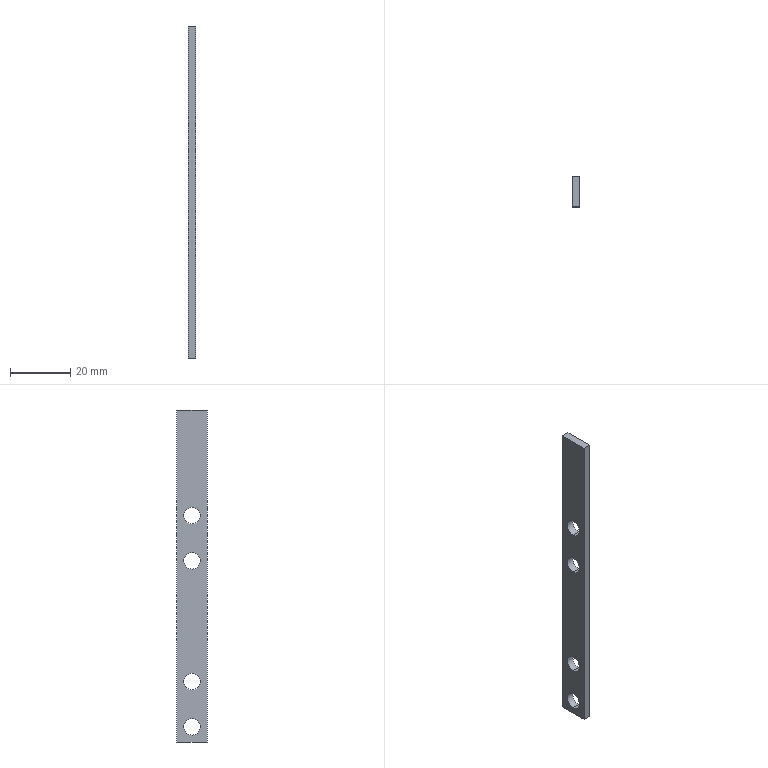Part | SolidWorks | features BaseBody 1 | 1 solid | 14 faces | box 2.5 x 10 x 110 mm | volume 2512 mm3 | cylinder 8 | plane 6 | commonest cylinder face diameters 5.5 x8
STEP:
#1=CARTESIAN_POINT('',(944.446,-4365.973,912.221));
#2=VERTEX_POINT('',#1);
#3=CARTESIAN_POINT('',(944.446,-4365.973,917.721));
#4=VERTEX_POINT('',#3);
#5=CARTESIAN_POINT('',(944.446,-4365.973,914.971));
#6=DIRECTION('',(-1.,0.,0.));
#7=DIRECTION('',(0.,0.,1.));
#8=AXIS2_PLACEMENT_3D('',#5,#6,#7);
#9=CIRCLE('',#8,2.75);
#10=EDGE_CURVE('',#2,#4,#9,.T.);
#11=ORIENTED_EDGE('',*,*,#10,.F.);
#12=CARTESIAN_POINT('',(941.946,-4365.973,912.221));
#13=VERTEX_POINT('',#12);
#14=CARTESIAN_POINT('',(882.499,-4365.973,912.221));
#15=DIRECTION('',(-1.,0.,0.));
#16=VECTOR('',#15,1000.);
#17=LINE('',#14,#16);
#18=EDGE_CURVE('',#2,#13,#17,.T.);
#19=ORIENTED_EDGE('',*,*,#18,.T.);
#20=CARTESIAN_POINT('',(941.946,-4365.973,917.721));
#21=VERTEX_POINT('',#20);
#22=CARTESIAN_POINT('',(941.946,-4365.973,914.971));
#23=DIRECTION('',(1.,0.,0.));
#24=DIRECTION('',(0.,0.,1.));
#25=AXIS2_PLACEMENT_3D('',#22,#23,#24);
#26=CIRCLE('',#25,2.75);
#27=EDGE_CURVE('',#21,#13,#26,.T.);
#28=ORIENTED_EDGE('',*,*,#27,.F.);
#29=CARTESIAN_POINT('',(882.499,-4365.973,917.721));
#30=DIRECTION('',(-1.,0.,0.));
#31=VECTOR('',#30,1000.);
#32=LINE('',#29,#31);
#33=EDGE_CURVE('',#4,#21,#32,.T.);
#34=ORIENTED_EDGE('',*,*,#33,.F.);
#35=EDGE_LOOP('',(#11,#19,#28,#34));
#36=FACE_OUTER_BOUND('',#35,.T.);
#37=CARTESIAN_POINT('',(882.499,-4365.973,914.971));
#38=DIRECTION('',(-1.,0.,0.));
#39=DIRECTION('',(0.,0.,1.));
#40=AXIS2_PLACEMENT_3D('',#37,#38,#39);
#41=CYLINDRICAL_SURFACE('',#40,2.75);
#42=ADVANCED_FACE('',(#36),#41,.F.);
#43=CARTESIAN_POINT('',(941.946,-4365.973,877.721));
#44=VERTEX_POINT('',#43);
#45=CARTESIAN_POINT('',(941.946,-4365.973,872.221));
#46=VERTEX_POINT('',#45);
#47=CARTESIAN_POINT('',(941.946,-4365.973,874.971));
#48=DIRECTION('',(1.,0.,0.));
#49=DIRECTION('',(0.,0.,-1.));
#50=AXIS2_PLACEMENT_3D('',#47,#48,#49);
#51=CIRCLE('',#50,2.75);
#52=EDGE_CURVE('',#44,#46,#51,.T.);
#53=ORIENTED_EDGE('',*,*,#52,.F.);
#54=CARTESIAN_POINT('',(944.446,-4365.973,877.721));
#55=VERTEX_POINT('',#54);
#56=CARTESIAN_POINT('',(882.499,-4365.973,877.721));
#57=DIRECTION('',(1.,0.,0.));
#58=VECTOR('',#57,1000.);
#59=LINE('',#56,#58);
#60=EDGE_CURVE('',#44,#55,#59,.T.);
#61=ORIENTED_EDGE('',*,*,#60,.T.);
#62=CARTESIAN_POINT('',(944.446,-4365.973,872.221));
#63=VERTEX_POINT('',#62);
#64=CARTESIAN_POINT('',(944.446,-4365.973,874.971));
#65=DIRECTION('',(-1.,0.,0.));
#66=DIRECTION('',(0.,0.,-1.));
#67=AXIS2_PLACEMENT_3D('',#64,#65,#66);
#68=CIRCLE('',#67,2.75);
#69=EDGE_CURVE('',#63,#55,#68,.T.);
#70=ORIENTED_EDGE('',*,*,#69,.F.);
#71=CARTESIAN_POINT('',(882.499,-4365.973,872.221));
#72=DIRECTION('',(1.,0.,0.));
#73=VECTOR('',#72,1000.);
#74=LINE('',#71,#73);
#75=EDGE_CURVE('',#46,#63,#74,.T.);
#76=ORIENTED_EDGE('',*,*,#75,.F.);
#77=EDGE_LOOP('',(#53,#61,#70,#76));
#78=FACE_OUTER_BOUND('',#77,.T.);
#79=CARTESIAN_POINT('',(882.499,-4365.973,874.971));
#80=DIRECTION('',(1.,0.,0.));
#81=DIRECTION('',(0.,0.,-1.));
#82=AXIS2_PLACEMENT_3D('',#79,#80,#81);
#83=CYLINDRICAL_SURFACE('',#82,2.75);
#84=ADVANCED_FACE('',(#78),#83,.F.);
#85=CARTESIAN_POINT('',(941.946,-4365.973,862.721));
#86=VERTEX_POINT('',#85);
#87=CARTESIAN_POINT('',(941.946,-4365.973,857.221));
#88=VERTEX_POINT('',#87);
#89=CARTESIAN_POINT('',(941.946,-4365.973,859.971));
#90=DIRECTION('',(1.,0.,0.));
#91=DIRECTION('',(0.,0.,-1.));
#92=AXIS2_PLACEMENT_3D('',#89,#90,#91);
#93=CIRCLE('',#92,2.75);
#94=EDGE_CURVE('',#86,#88,#93,.T.);
#95=ORIENTED_EDGE('',*,*,#94,.F.);
#96=CARTESIAN_POINT('',(944.446,-4365.973,862.721));
#97=VERTEX_POINT('',#96);
#98=CARTESIAN_POINT('',(882.499,-4365.973,862.721));
#99=DIRECTION('',(1.,0.,0.));
#100=VECTOR('',#99,1000.);
#101=LINE('',#98,#100);
#102=EDGE_CURVE('',#86,#97,#101,.T.);
#103=ORIENTED_EDGE('',*,*,#102,.T.);
#104=CARTESIAN_POINT('',(944.446,-4365.973,857.221));
#105=VERTEX_POINT('',#104);
#106=CARTESIAN_POINT('',(944.446,-4365.973,859.971));
#107=DIRECTION('',(-1.,0.,0.));
#108=DIRECTION('',(0.,0.,-1.));
#109=AXIS2_PLACEMENT_3D('',#106,#107,#108);
#110=CIRCLE('',#109,2.75);
#111=EDGE_CURVE('',#105,#97,#110,.T.);
#112=ORIENTED_EDGE('',*,*,#111,.F.);
#113=CARTESIAN_POINT('',(882.499,-4365.973,857.221));
#114=DIRECTION('',(1.,0.,0.));
#115=VECTOR('',#114,1000.);
#116=LINE('',#113,#115);
#117=EDGE_CURVE('',#88,#105,#116,.T.);
#118=ORIENTED_EDGE('',*,*,#117,.F.);
#119=EDGE_LOOP('',(#95,#103,#112,#118));
#120=FACE_OUTER_BOUND('',#119,.T.);
#121=CARTESIAN_POINT('',(882.499,-4365.973,859.971));
#122=DIRECTION('',(1.,0.,0.));
#123=DIRECTION('',(0.,0.,-1.));
#124=AXIS2_PLACEMENT_3D('',#121,#122,#123);
#125=CYLINDRICAL_SURFACE('',#124,2.75);
#126=ADVANCED_FACE('',(#120),#125,.F.);
#127=CARTESIAN_POINT('',(944.446,-4365.973,927.221));
#128=VERTEX_POINT('',#127);
#129=CARTESIAN_POINT('',(944.446,-4365.973,932.721));
#130=VERTEX_POINT('',#129);
#131=CARTESIAN_POINT('',(944.446,-4365.973,929.971));
#132=DIRECTION('',(-1.,0.,0.));
#133=DIRECTION('',(0.,0.,1.));
#134=AXIS2_PLACEMENT_3D('',#131,#132,#133);
#135=CIRCLE('',#134,2.75);
#136=EDGE_CURVE('',#128,#130,#135,.T.);
#137=ORIENTED_EDGE('',*,*,#136,.F.);
#138=CARTESIAN_POINT('',(941.946,-4365.973,927.221));
#139=VERTEX_POINT('',#138);
#140=CARTESIAN_POINT('',(882.499,-4365.973,927.221));
#141=DIRECTION('',(-1.,0.,0.));
#142=VECTOR('',#141,1000.);
#143=LINE('',#140,#142);
#144=EDGE_CURVE('',#128,#139,#143,.T.);
#145=ORIENTED_EDGE('',*,*,#144,.T.);
#146=CARTESIAN_POINT('',(941.946,-4365.973,932.721));
#147=VERTEX_POINT('',#146);
#148=CARTESIAN_POINT('',(941.946,-4365.973,929.971));
#149=DIRECTION('',(1.,0.,0.));
#150=DIRECTION('',(0.,0.,1.));
#151=AXIS2_PLACEMENT_3D('',#148,#149,#150);
#152=CIRCLE('',#151,2.75);
#153=EDGE_CURVE('',#147,#139,#152,.T.);
#154=ORIENTED_EDGE('',*,*,#153,.F.);
#155=CARTESIAN_POINT('',(882.499,-4365.973,932.721));
#156=DIRECTION('',(-1.,0.,0.));
#157=VECTOR('',#156,1000.);
#158=LINE('',#155,#157);
#159=EDGE_CURVE('',#130,#147,#158,.T.);
#160=ORIENTED_EDGE('',*,*,#159,.F.);
#161=EDGE_LOOP('',(#137,#145,#154,#160));
#162=FACE_OUTER_BOUND('',#161,.T.);
#163=CARTESIAN_POINT('',(882.499,-4365.973,929.971));
#164=DIRECTION('',(-1.,0.,0.));
#165=DIRECTION('',(0.,0.,1.));
#166=AXIS2_PLACEMENT_3D('',#163,#164,#165);
#167=CYLINDRICAL_SURFACE('',#166,2.75);
#168=ADVANCED_FACE('',(#162),#167,.F.);
#169=CARTESIAN_POINT('',(941.946,-4360.973,854.971));
#170=VERTEX_POINT('',#169);
#171=CARTESIAN_POINT('',(941.946,-4370.973,854.971));
#172=VERTEX_POINT('',#171);
#173=CARTESIAN_POINT('',(941.946,-4370.973,854.971));
#174=DIRECTION('',(0.,-1.,0.));
#175=VECTOR('',#174,1000.);
#176=LINE('',#173,#175);
#177=EDGE_CURVE('',#170,#172,#176,.T.);
#178=ORIENTED_EDGE('',*,*,#177,.T.);
#179=CARTESIAN_POINT('',(941.946,-4370.973,964.971));
#180=VERTEX_POINT('',#179);
#181=CARTESIAN_POINT('',(941.946,-4370.973,854.971));
#182=DIRECTION('',(0.,0.,1.));
#183=VECTOR('',#182,1000.);
#184=LINE('',#181,#183);
#185=EDGE_CURVE('',#172,#180,#184,.T.);
#186=ORIENTED_EDGE('',*,*,#185,.T.);
#187=CARTESIAN_POINT('',(941.946,-4360.973,964.971));
#188=VERTEX_POINT('',#187);
#189=CARTESIAN_POINT('',(941.946,-4370.973,964.971));
#190=DIRECTION('',(0.,1.,0.));
#191=VECTOR('',#190,1000.);
#192=LINE('',#189,#191);
#193=EDGE_CURVE('',#180,#188,#192,.T.);
#194=ORIENTED_EDGE('',*,*,#193,.T.);
#195=CARTESIAN_POINT('',(941.946,-4360.973,854.971));
#196=DIRECTION('',(0.,0.,-1.));
#197=VECTOR('',#196,1000.);
#198=LINE('',#195,#197);
#199=EDGE_CURVE('',#188,#170,#198,.T.);
#200=ORIENTED_EDGE('',*,*,#199,.T.);
#201=EDGE_LOOP('',(#178,#186,#194,#200));
#202=FACE_OUTER_BOUND('',#201,.T.);
#203=ORIENTED_EDGE('',*,*,#27,.T.);
#204=CARTESIAN_POINT('',(941.946,-4365.973,914.971));
#205=DIRECTION('',(1.,0.,0.));
#206=DIRECTION('',(0.,0.,1.));
#207=AXIS2_PLACEMENT_3D('',#204,#205,#206);
#208=CIRCLE('',#207,2.75);
#209=EDGE_CURVE('',#13,#21,#208,.T.);
#210=ORIENTED_EDGE('',*,*,#209,.T.);
#211=EDGE_LOOP('',(#203,#210));
#212=FACE_BOUND('',#211,.T.);
#213=CARTESIAN_POINT('',(941.946,-4365.973,874.971));
#214=DIRECTION('',(1.,0.,0.));
#215=DIRECTION('',(0.,0.,-1.));
#216=AXIS2_PLACEMENT_3D('',#213,#214,#215);
#217=CIRCLE('',#216,2.75);
#218=EDGE_CURVE('',#46,#44,#217,.T.);
#219=ORIENTED_EDGE('',*,*,#218,.T.);
#220=ORIENTED_EDGE('',*,*,#52,.T.);
#221=EDGE_LOOP('',(#219,#220));
#222=FACE_BOUND('',#221,.T.);
#223=CARTESIAN_POINT('',(941.946,-4365.973,859.971));
#224=DIRECTION('',(1.,0.,0.));
#225=DIRECTION('',(0.,0.,-1.));
#226=AXIS2_PLACEMENT_3D('',#223,#224,#225);
#227=CIRCLE('',#226,2.75);
#228=EDGE_CURVE('',#88,#86,#227,.T.);
#229=ORIENTED_EDGE('',*,*,#228,.T.);
#230=ORIENTED_EDGE('',*,*,#94,.T.);
#231=EDGE_LOOP('',(#229,#230));
#232=FACE_BOUND('',#231,.T.);
#233=ORIENTED_EDGE('',*,*,#153,.T.);
#234=CARTESIAN_POINT('',(941.946,-4365.973,929.971));
#235=DIRECTION('',(1.,0.,0.));
#236=DIRECTION('',(0.,0.,1.));
#237=AXIS2_PLACEMENT_3D('',#234,#235,#236);
#238=CIRCLE('',#237,2.75);
#239=EDGE_CURVE('',#139,#147,#238,.T.);
#240=ORIENTED_EDGE('',*,*,#239,.T.);
#241=EDGE_LOOP('',(#233,#240));
#242=FACE_BOUND('',#241,.T.);
#243=CARTESIAN_POINT('',(941.946,-4370.973,854.971));
#244=DIRECTION('',(-1.,0.,0.));
#245=DIRECTION('',(0.,0.,1.));
#246=AXIS2_PLACEMENT_3D('',#243,#244,#245);
#247=PLANE('',#246);
#248=ADVANCED_FACE('',(#202,#212,#222,#232,#242),#247,.T.);
#249=CARTESIAN_POINT('',(944.446,-4370.973,854.971));
#250=VERTEX_POINT('',#249);
#251=CARTESIAN_POINT('',(944.446,-4370.973,854.971));
#252=DIRECTION('',(1.,0.,0.));
#253=VECTOR('',#252,1000.);
#254=LINE('',#251,#253);
#255=EDGE_CURVE('',#172,#250,#254,.T.);
#256=ORIENTED_EDGE('',*,*,#255,.T.);
#257=CARTESIAN_POINT('',(944.446,-4370.973,964.971));
#258=VERTEX_POINT('',#257);
#259=CARTESIAN_POINT('',(944.446,-4370.973,854.971));
#260=DIRECTION('',(0.,0.,1.));
#261=VECTOR('',#260,1000.);
#262=LINE('',#259,#261);
#263=EDGE_CURVE('',#250,#258,#262,.T.);
#264=ORIENTED_EDGE('',*,*,#263,.T.);
#265=CARTESIAN_POINT('',(944.446,-4370.973,964.971));
#266=DIRECTION('',(-1.,0.,0.));
#267=VECTOR('',#266,1000.);
#268=LINE('',#265,#267);
#269=EDGE_CURVE('',#258,#180,#268,.T.);
#270=ORIENTED_EDGE('',*,*,#269,.T.);
#271=ORIENTED_EDGE('',*,*,#185,.F.);
#272=EDGE_LOOP('',(#256,#264,#270,#271));
#273=FACE_OUTER_BOUND('',#272,.T.);
#274=CARTESIAN_POINT('',(944.446,-4370.973,854.971));
#275=DIRECTION('',(0.,-1.,0.));
#276=DIRECTION('',(0.,0.,-1.));
#277=AXIS2_PLACEMENT_3D('',#274,#275,#276);
#278=PLANE('',#277);
#279=ADVANCED_FACE('',(#273),#278,.T.);
#280=ORIENTED_EDGE('',*,*,#177,.F.);
#281=CARTESIAN_POINT('',(944.446,-4360.973,854.971));
#282=VERTEX_POINT('',#281);
#283=CARTESIAN_POINT('',(943.196,-4360.973,854.971));
#284=DIRECTION('',(-1.,0.,0.));
#285=VECTOR('',#284,1000.);
#286=LINE('',#283,#285);
#287=EDGE_CURVE('',#282,#170,#286,.T.);
#288=ORIENTED_EDGE('',*,*,#287,.F.);
#289=CARTESIAN_POINT('',(944.446,-4365.973,854.971));
#290=DIRECTION('',(0.,1.,0.));
#291=VECTOR('',#290,1000.);
#292=LINE('',#289,#291);
#293=EDGE_CURVE('',#250,#282,#292,.T.);
#294=ORIENTED_EDGE('',*,*,#293,.F.);
#295=ORIENTED_EDGE('',*,*,#255,.F.);
#296=EDGE_LOOP('',(#280,#288,#294,#295));
#297=FACE_OUTER_BOUND('',#296,.T.);
#298=CARTESIAN_POINT('',(943.196,-4365.973,854.971));
#299=DIRECTION('',(0.,0.,1.));
#300=DIRECTION('',(1.,0.,0.));
#301=AXIS2_PLACEMENT_3D('',#298,#299,#300);
#302=PLANE('',#301);
#303=ADVANCED_FACE('',(#297),#302,.F.);
#304=ORIENTED_EDGE('',*,*,#287,.T.);
#305=ORIENTED_EDGE('',*,*,#199,.F.);
#306=CARTESIAN_POINT('',(944.446,-4360.973,964.971));
#307=VERTEX_POINT('',#306);
#308=CARTESIAN_POINT('',(941.946,-4360.973,964.971));
#309=DIRECTION('',(1.,0.,0.));
#310=VECTOR('',#309,1000.);
#311=LINE('',#308,#310);
#312=EDGE_CURVE('',#188,#307,#311,.T.);
#313=ORIENTED_EDGE('',*,*,#312,.T.);
#314=CARTESIAN_POINT('',(944.446,-4360.973,854.971));
#315=DIRECTION('',(0.,0.,-1.));
#316=VECTOR('',#315,1000.);
#317=LINE('',#314,#316);
#318=EDGE_CURVE('',#307,#282,#317,.T.);
#319=ORIENTED_EDGE('',*,*,#318,.T.);
#320=EDGE_LOOP('',(#304,#305,#313,#319));
#321=FACE_OUTER_BOUND('',#320,.T.);
#322=CARTESIAN_POINT('',(941.946,-4360.973,854.971));
#323=DIRECTION('',(0.,1.,0.));
#324=DIRECTION('',(0.,0.,1.));
#325=AXIS2_PLACEMENT_3D('',#322,#323,#324);
#326=PLANE('',#325);
#327=ADVANCED_FACE('',(#321),#326,.T.);
#328=CARTESIAN_POINT('',(944.446,-4365.973,964.971));
#329=DIRECTION('',(0.,1.,0.));
#330=VECTOR('',#329,1000.);
#331=LINE('',#328,#330);
#332=EDGE_CURVE('',#258,#307,#331,.T.);
#333=ORIENTED_EDGE('',*,*,#332,.T.);
#334=ORIENTED_EDGE('',*,*,#312,.F.);
#335=ORIENTED_EDGE('',*,*,#193,.F.);
#336=ORIENTED_EDGE('',*,*,#269,.F.);
#337=EDGE_LOOP('',(#333,#334,#335,#336));
#338=FACE_OUTER_BOUND('',#337,.T.);
#339=CARTESIAN_POINT('',(943.196,-4365.973,964.971));
#340=DIRECTION('',(0.,0.,1.));
#341=DIRECTION('',(1.,0.,0.));
#342=AXIS2_PLACEMENT_3D('',#339,#340,#341);
#343=PLANE('',#342);
#344=ADVANCED_FACE('',(#338),#343,.T.);
#345=ORIENTED_EDGE('',*,*,#18,.F.);
#346=CARTESIAN_POINT('',(944.446,-4365.973,914.971));
#347=DIRECTION('',(-1.,0.,0.));
#348=DIRECTION('',(0.,0.,1.));
#349=AXIS2_PLACEMENT_3D('',#346,#347,#348);
#350=CIRCLE('',#349,2.75);
#351=EDGE_CURVE('',#4,#2,#350,.T.);
#352=ORIENTED_EDGE('',*,*,#351,.F.);
#353=ORIENTED_EDGE('',*,*,#33,.T.);
#354=ORIENTED_EDGE('',*,*,#209,.F.);
#355=EDGE_LOOP('',(#345,#352,#353,#354));
#356=FACE_OUTER_BOUND('',#355,.T.);
#357=CARTESIAN_POINT('',(882.499,-4365.973,914.971));
#358=DIRECTION('',(-1.,0.,0.));
#359=DIRECTION('',(0.,0.,1.));
#360=AXIS2_PLACEMENT_3D('',#357,#358,#359);
#361=CYLINDRICAL_SURFACE('',#360,2.75);
#362=ADVANCED_FACE('',(#356),#361,.F.);
#363=ORIENTED_EDGE('',*,*,#60,.F.);
#364=ORIENTED_EDGE('',*,*,#218,.F.);
#365=ORIENTED_EDGE('',*,*,#75,.T.);
#366=CARTESIAN_POINT('',(944.446,-4365.973,874.971));
#367=DIRECTION('',(-1.,0.,0.));
#368=DIRECTION('',(0.,0.,-1.));
#369=AXIS2_PLACEMENT_3D('',#366,#367,#368);
#370=CIRCLE('',#369,2.75);
#371=EDGE_CURVE('',#55,#63,#370,.T.);
#372=ORIENTED_EDGE('',*,*,#371,.F.);
#373=EDGE_LOOP('',(#363,#364,#365,#372));
#374=FACE_OUTER_BOUND('',#373,.T.);
#375=CARTESIAN_POINT('',(882.499,-4365.973,874.971));
#376=DIRECTION('',(1.,0.,0.));
#377=DIRECTION('',(0.,0.,-1.));
#378=AXIS2_PLACEMENT_3D('',#375,#376,#377);
#379=CYLINDRICAL_SURFACE('',#378,2.75);
#380=ADVANCED_FACE('',(#374),#379,.F.);
#381=ORIENTED_EDGE('',*,*,#102,.F.);
#382=ORIENTED_EDGE('',*,*,#228,.F.);
#383=ORIENTED_EDGE('',*,*,#117,.T.);
#384=CARTESIAN_POINT('',(944.446,-4365.973,859.971));
#385=DIRECTION('',(-1.,0.,0.));
#386=DIRECTION('',(0.,0.,-1.));
#387=AXIS2_PLACEMENT_3D('',#384,#385,#386);
#388=CIRCLE('',#387,2.75);
#389=EDGE_CURVE('',#97,#105,#388,.T.);
#390=ORIENTED_EDGE('',*,*,#389,.F.);
#391=EDGE_LOOP('',(#381,#382,#383,#390));
#392=FACE_OUTER_BOUND('',#391,.T.);
#393=CARTESIAN_POINT('',(882.499,-4365.973,859.971));
#394=DIRECTION('',(1.,0.,0.));
#395=DIRECTION('',(0.,0.,-1.));
#396=AXIS2_PLACEMENT_3D('',#393,#394,#395);
#397=CYLINDRICAL_SURFACE('',#396,2.75);
#398=ADVANCED_FACE('',(#392),#397,.F.);
#399=ORIENTED_EDGE('',*,*,#144,.F.);
#400=CARTESIAN_POINT('',(944.446,-4365.973,929.971));
#401=DIRECTION('',(-1.,0.,0.));
#402=DIRECTION('',(0.,0.,1.));
#403=AXIS2_PLACEMENT_3D('',#400,#401,#402);
#404=CIRCLE('',#403,2.75);
#405=EDGE_CURVE('',#130,#128,#404,.T.);
#406=ORIENTED_EDGE('',*,*,#405,.F.);
#407=ORIENTED_EDGE('',*,*,#159,.T.);
#408=ORIENTED_EDGE('',*,*,#239,.F.);
#409=EDGE_LOOP('',(#399,#406,#407,#408));
#410=FACE_OUTER_BOUND('',#409,.T.);
#411=CARTESIAN_POINT('',(882.499,-4365.973,929.971));
#412=DIRECTION('',(-1.,0.,0.));
#413=DIRECTION('',(0.,0.,1.));
#414=AXIS2_PLACEMENT_3D('',#411,#412,#413);
#415=CYLINDRICAL_SURFACE('',#414,2.75);
#416=ADVANCED_FACE('',(#410),#415,.F.);
#417=ORIENTED_EDGE('',*,*,#293,.T.);
#418=ORIENTED_EDGE('',*,*,#318,.F.);
#419=ORIENTED_EDGE('',*,*,#332,.F.);
#420=ORIENTED_EDGE('',*,*,#263,.F.);
#421=EDGE_LOOP('',(#417,#418,#419,#420));
#422=FACE_OUTER_BOUND('',#421,.T.);
#423=ORIENTED_EDGE('',*,*,#351,.T.);
#424=ORIENTED_EDGE('',*,*,#10,.T.);
#425=EDGE_LOOP('',(#423,#424));
#426=FACE_BOUND('',#425,.T.);
#427=ORIENTED_EDGE('',*,*,#69,.T.);
#428=ORIENTED_EDGE('',*,*,#371,.T.);
#429=EDGE_LOOP('',(#427,#428));
#430=FACE_BOUND('',#429,.T.);
#431=ORIENTED_EDGE('',*,*,#111,.T.);
#432=ORIENTED_EDGE('',*,*,#389,.T.);
#433=EDGE_LOOP('',(#431,#432));
#434=FACE_BOUND('',#433,.T.);
#435=ORIENTED_EDGE('',*,*,#405,.T.);
#436=ORIENTED_EDGE('',*,*,#136,.T.);
#437=EDGE_LOOP('',(#435,#436));
#438=FACE_BOUND('',#437,.T.);
#439=CARTESIAN_POINT('',(944.446,-4360.973,854.971));
#440=DIRECTION('',(1.,0.,0.));
#441=DIRECTION('',(0.,0.,-1.));
#442=AXIS2_PLACEMENT_3D('',#439,#440,#441);
#443=PLANE('',#442);
#444=ADVANCED_FACE('',(#422,#426,#430,#434,#438),#443,.T.);
#445=CLOSED_SHELL('',(#42,#84,#126,#168,#248,#279,#303,#327,#344,#362,#380,#398,#416,#444));
#446=MANIFOLD_SOLID_BREP('',#445);
#447=CARTESIAN_POINT('',(0.,0.,0.));
#448=DIRECTION('',(0.,0.,1.));
#449=DIRECTION('',(1.,0.,0.));
#450=AXIS2_PLACEMENT_3D('',#447,#448,#449);
#451=(LENGTH_UNIT()NAMED_UNIT(*)SI_UNIT(.MILLI.,.METRE.));
#452=UNCERTAINTY_MEASURE_WITH_UNIT(LENGTH_MEASURE(0.00001),#451,'','');
#453=(NAMED_UNIT(*)PLANE_ANGLE_UNIT()SI_UNIT($,.RADIAN.));
#454=(NAMED_UNIT(*)SI_UNIT($,.STERADIAN.)SOLID_ANGLE_UNIT());
#455=(GEOMETRIC_REPRESENTATION_CONTEXT(3)GLOBAL_UNCERTAINTY_ASSIGNED_CONTEXT((#452))GLOBAL_UNIT_ASSIGNED_CONTEXT((#451,#453,#454))REPRESENTATION_CONTEXT('',''));
#456=ADVANCED_BREP_SHAPE_REPRESENTATION('',(#446,#450),#455);